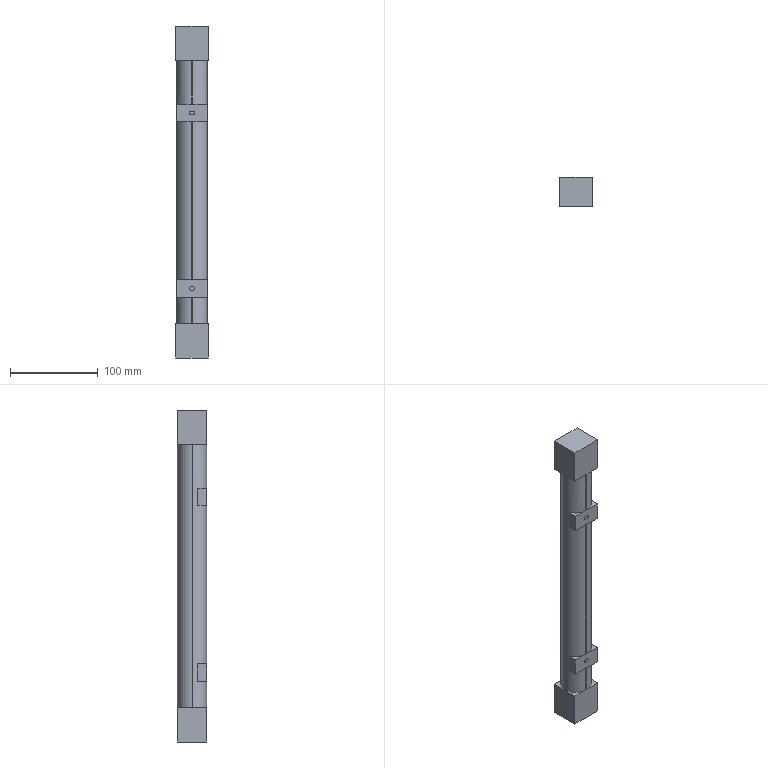Part | STEP file | LED lighting lamp QELTS-300-220 220V 300mm | 1 solid | 51 faces | box 37 x 33.2 x 378 mm | volume 378498 mm3 | plane 43 | cylinder 7 | spline 1 | commonest cylinder face diameters 4.2 x4 33.2 x3